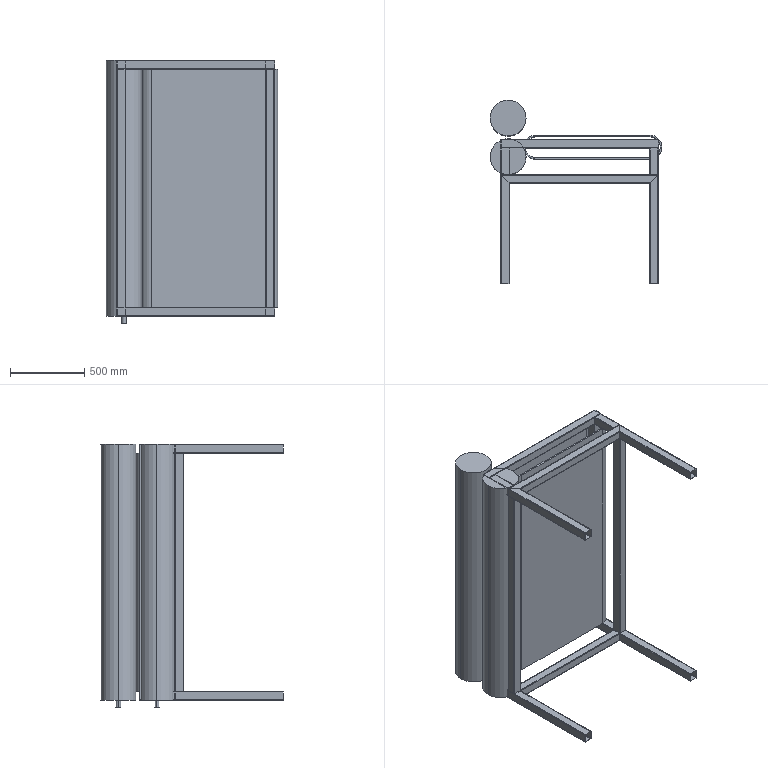Part | STEP file | Roller line_Default<Machined> | 21 solids | 316 faces | box 1152 x 1230 x 1771 mm | volume 196274753 mm3 | plane 174 | cylinder 142 | commonest cylinder face diameters 4 x64 8 x64 240 x4 141.191 x3 161.191 x3 30.257 x2